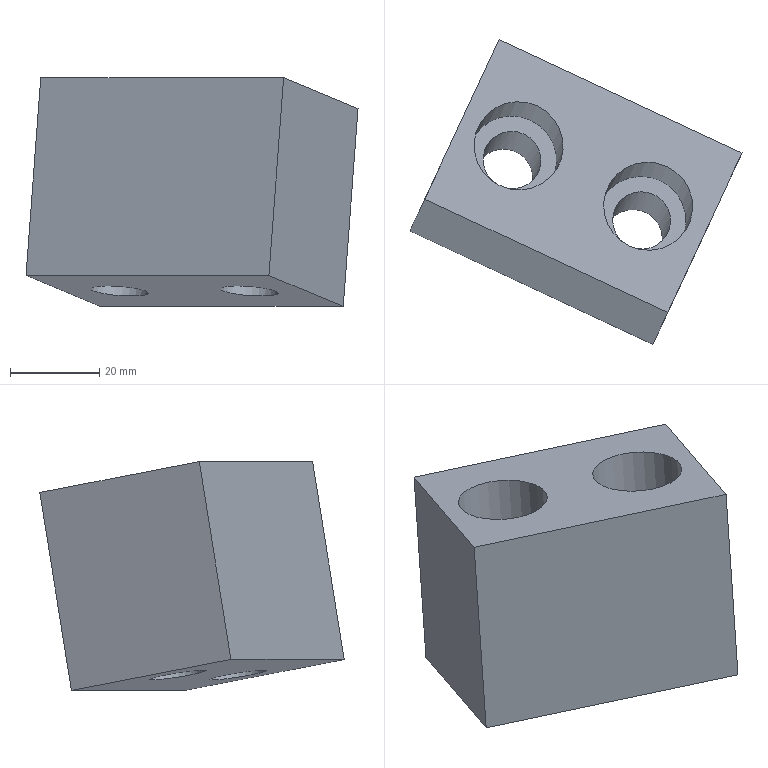Part | NX | features solid 2 | 1 solid | 12 faces | box 74.329 x 68.141 x 51.262 mm | volume 88797 mm3 | plane 8 | cylinder 4 | commonest cylinder face diameters 13 x2 20 x2
STEP:
#1=CARTESIAN_POINT('',(315.95,683.902,73.039));
#2=VERTEX_POINT('',#1);
#3=CARTESIAN_POINT('',(317.057,677.565,73.969));
#4=DIRECTION('',(-0.07339,-0.1574,-0.9848));
#5=DIRECTION('',(-0.1704,0.9749,-0.1431));
#6=AXIS2_PLACEMENT_3D('',#3,#4,#5);
#7=CIRCLE('',#6,6.5);
#8=EDGE_CURVE('',#2,#2,#7,.F.);
#9=ORIENTED_EDGE('',*,*,#8,.T.);
#10=EDGE_LOOP('',(#9));
#11=FACE_BOUND('',#10,.T.);
#12=CARTESIAN_POINT('',(286.948,697.426,73.039));
#13=VERTEX_POINT('',#12);
#14=CARTESIAN_POINT('',(288.055,691.089,73.969));
#15=DIRECTION('',(-0.07339,-0.1574,-0.9848));
#16=DIRECTION('',(-0.1704,0.9749,-0.1431));
#17=AXIS2_PLACEMENT_3D('',#14,#15,#16);
#18=CIRCLE('',#17,6.5);
#19=EDGE_CURVE('',#13,#13,#18,.F.);
#20=ORIENTED_EDGE('',*,*,#19,.T.);
#21=EDGE_LOOP('',(#20));
#22=FACE_BOUND('',#21,.T.);
#23=CARTESIAN_POINT('',(267.043,679.155,77.442));
#24=VERTEX_POINT('',#23);
#25=CARTESIAN_POINT('',(283.691,714.857,70.496));
#26=VERTEX_POINT('',#25);
#27=CARTESIAN_POINT('',(267.043,679.155,77.442));
#28=DIRECTION('',(0.4162,0.8925,-0.1736));
#29=VECTOR('',#28,1000.);
#30=LINE('',#27,#29);
#31=EDGE_CURVE('',#24,#26,#30,.T.);
#32=ORIENTED_EDGE('',*,*,#31,.T.);
#33=CARTESIAN_POINT('',(338.07,689.499,70.496));
#34=VERTEX_POINT('',#33);
#35=CARTESIAN_POINT('',(338.07,689.499,70.496));
#36=DIRECTION('',(0.9063,-0.4226,0.));
#37=VECTOR('',#36,1000.);
#38=LINE('',#35,#37);
#39=EDGE_CURVE('',#34,#26,#38,.F.);
#40=ORIENTED_EDGE('',*,*,#39,.F.);
#41=CARTESIAN_POINT('',(321.422,653.798,77.442));
#42=VERTEX_POINT('',#41);
#43=CARTESIAN_POINT('',(321.422,653.798,77.442));
#44=DIRECTION('',(-0.4162,-0.8925,0.1736));
#45=VECTOR('',#44,1000.);
#46=LINE('',#43,#45);
#47=EDGE_CURVE('',#42,#34,#46,.F.);
#48=ORIENTED_EDGE('',*,*,#47,.F.);
#49=CARTESIAN_POINT('',(321.422,653.798,77.442));
#50=DIRECTION('',(0.9063,-0.4226,0.));
#51=VECTOR('',#50,1000.);
#52=LINE('',#49,#51);
#53=EDGE_CURVE('',#42,#24,#52,.F.);
#54=ORIENTED_EDGE('',*,*,#53,.T.);
#55=EDGE_LOOP('',(#32,#40,#48,#54));
#56=FACE_BOUND('',#55,.T.);
#57=CARTESIAN_POINT('',(321.422,653.798,77.442));
#58=DIRECTION('',(-0.07339,-0.1574,-0.9848));
#59=DIRECTION('',(-0.9063,0.4226,0.));
#60=AXIS2_PLACEMENT_3D('',#57,#58,#59);
#61=PLANE('',#60);
#62=ADVANCED_FACE('',(#11,#22,#56),#61,.T.);
#63=ORIENTED_EDGE('',*,*,#47,.T.);
#64=CARTESIAN_POINT('',(341.372,696.581,114.812));
#65=VERTEX_POINT('',#64);
#66=CARTESIAN_POINT('',(336.969,687.139,55.724));
#67=DIRECTION('',(-0.07339,-0.1574,-0.9848));
#68=VECTOR('',#67,1000.);
#69=LINE('',#66,#68);
#70=EDGE_CURVE('',#34,#65,#69,.F.);
#71=ORIENTED_EDGE('',*,*,#70,.T.);
#72=CARTESIAN_POINT('',(324.724,660.88,121.758));
#73=VERTEX_POINT('',#72);
#74=CARTESIAN_POINT('',(324.724,660.88,121.758));
#75=DIRECTION('',(0.4162,0.8925,-0.1736));
#76=VECTOR('',#75,1000.);
#77=LINE('',#74,#76);
#78=EDGE_CURVE('',#73,#65,#77,.T.);
#79=ORIENTED_EDGE('',*,*,#78,.F.);
#80=CARTESIAN_POINT('',(320.321,651.437,62.67));
#81=DIRECTION('',(0.07339,0.1574,0.9848));
#82=VECTOR('',#81,1000.);
#83=LINE('',#80,#82);
#84=EDGE_CURVE('',#42,#73,#83,.T.);
#85=ORIENTED_EDGE('',*,*,#84,.F.);
#86=EDGE_LOOP('',(#63,#71,#79,#85));
#87=FACE_BOUND('',#86,.T.);
#88=CARTESIAN_POINT('',(320.321,651.437,62.67));
#89=DIRECTION('',(-0.9063,0.4226,0.));
#90=DIRECTION('',(0.07339,0.1574,0.9848));
#91=AXIS2_PLACEMENT_3D('',#88,#89,#90);
#92=PLANE('',#91);
#93=ADVANCED_FACE('',(#87),#92,.F.);
#94=CARTESIAN_POINT('',(316.198,675.722,120.022));
#95=VERTEX_POINT('',#94);
#96=CARTESIAN_POINT('',(320.36,684.647,118.285));
#97=DIRECTION('',(-0.07339,-0.1574,-0.9848));
#98=DIRECTION('',(-0.4162,-0.8925,0.1736));
#99=AXIS2_PLACEMENT_3D('',#96,#97,#98);
#100=CIRCLE('',#99,10.);
#101=EDGE_CURVE('',#95,#95,#100,.T.);
#102=ORIENTED_EDGE('',*,*,#101,.T.);
#103=EDGE_LOOP('',(#102));
#104=FACE_BOUND('',#103,.T.);
#105=CARTESIAN_POINT('',(287.196,689.246,120.022));
#106=VERTEX_POINT('',#105);
#107=CARTESIAN_POINT('',(291.358,698.171,118.285));
#108=DIRECTION('',(-0.07339,-0.1574,-0.9848));
#109=DIRECTION('',(-0.4162,-0.8925,0.1736));
#110=AXIS2_PLACEMENT_3D('',#107,#108,#109);
#111=CIRCLE('',#110,10.);
#112=EDGE_CURVE('',#106,#106,#111,.T.);
#113=ORIENTED_EDGE('',*,*,#112,.T.);
#114=EDGE_LOOP('',(#113));
#115=FACE_BOUND('',#114,.T.);
#116=ORIENTED_EDGE('',*,*,#78,.T.);
#117=CARTESIAN_POINT('',(286.993,721.939,114.812));
#118=VERTEX_POINT('',#117);
#119=CARTESIAN_POINT('',(341.372,696.581,114.812));
#120=DIRECTION('',(-0.9063,0.4226,0.));
#121=VECTOR('',#120,1000.);
#122=LINE('',#119,#121);
#123=EDGE_CURVE('',#65,#118,#122,.T.);
#124=ORIENTED_EDGE('',*,*,#123,.T.);
#125=CARTESIAN_POINT('',(270.346,686.237,121.758));
#126=VERTEX_POINT('',#125);
#127=CARTESIAN_POINT('',(270.346,686.237,121.758));
#128=DIRECTION('',(-0.4162,-0.8925,0.1736));
#129=VECTOR('',#128,1000.);
#130=LINE('',#127,#129);
#131=EDGE_CURVE('',#126,#118,#130,.F.);
#132=ORIENTED_EDGE('',*,*,#131,.F.);
#133=CARTESIAN_POINT('',(324.724,660.88,121.758));
#134=DIRECTION('',(-0.9063,0.4226,0.));
#135=VECTOR('',#134,1000.);
#136=LINE('',#133,#135);
#137=EDGE_CURVE('',#73,#126,#136,.T.);
#138=ORIENTED_EDGE('',*,*,#137,.F.);
#139=EDGE_LOOP('',(#116,#124,#132,#138));
#140=FACE_BOUND('',#139,.T.);
#141=CARTESIAN_POINT('',(324.724,660.88,121.758));
#142=DIRECTION('',(-0.07339,-0.1574,-0.9848));
#143=DIRECTION('',(-0.9063,0.4226,0.));
#144=AXIS2_PLACEMENT_3D('',#141,#142,#143);
#145=PLANE('',#144);
#146=ADVANCED_FACE('',(#104,#115,#140),#145,.F.);
#147=CARTESIAN_POINT('',(265.942,676.794,62.67));
#148=DIRECTION('',(0.07339,0.1574,0.9848));
#149=VECTOR('',#148,1000.);
#150=LINE('',#147,#149);
#151=EDGE_CURVE('',#24,#126,#150,.T.);
#152=ORIENTED_EDGE('',*,*,#151,.T.);
#153=ORIENTED_EDGE('',*,*,#131,.T.);
#154=CARTESIAN_POINT('',(282.59,712.496,55.724));
#155=DIRECTION('',(-0.07339,-0.1574,-0.9848));
#156=VECTOR('',#155,1000.);
#157=LINE('',#154,#156);
#158=EDGE_CURVE('',#26,#118,#157,.F.);
#159=ORIENTED_EDGE('',*,*,#158,.F.);
#160=ORIENTED_EDGE('',*,*,#31,.F.);
#161=EDGE_LOOP('',(#152,#153,#159,#160));
#162=FACE_BOUND('',#161,.T.);
#163=CARTESIAN_POINT('',(265.942,676.794,62.67));
#164=DIRECTION('',(-0.9063,0.4226,0.));
#165=DIRECTION('',(0.07339,0.1574,0.9848));
#166=AXIS2_PLACEMENT_3D('',#163,#164,#165);
#167=PLANE('',#166);
#168=ADVANCED_FACE('',(#162),#167,.T.);
#169=ORIENTED_EDGE('',*,*,#123,.F.);
#170=ORIENTED_EDGE('',*,*,#70,.F.);
#171=ORIENTED_EDGE('',*,*,#39,.T.);
#172=ORIENTED_EDGE('',*,*,#158,.T.);
#173=EDGE_LOOP('',(#169,#170,#171,#172));
#174=FACE_BOUND('',#173,.T.);
#175=CARTESIAN_POINT('',(336.969,687.139,55.724));
#176=DIRECTION('',(0.4162,0.8925,-0.1736));
#177=DIRECTION('',(-0.07339,-0.1574,-0.9848));
#178=AXIS2_PLACEMENT_3D('',#175,#176,#177);
#179=PLANE('',#178);
#180=ADVANCED_FACE('',(#174),#179,.T.);
#181=ORIENTED_EDGE('',*,*,#137,.T.);
#182=ORIENTED_EDGE('',*,*,#151,.F.);
#183=ORIENTED_EDGE('',*,*,#53,.F.);
#184=ORIENTED_EDGE('',*,*,#84,.T.);
#185=EDGE_LOOP('',(#181,#182,#183,#184));
#186=FACE_BOUND('',#185,.T.);
#187=CARTESIAN_POINT('',(320.321,651.437,62.67));
#188=DIRECTION('',(0.4162,0.8925,-0.1736));
#189=DIRECTION('',(-0.07339,-0.1574,-0.9848));
#190=AXIS2_PLACEMENT_3D('',#187,#188,#189);
#191=PLANE('',#190);
#192=ADVANCED_FACE('',(#186),#191,.F.);
#193=CARTESIAN_POINT('',(287.185,689.222,99.718));
#194=VERTEX_POINT('',#193);
#195=CARTESIAN_POINT('',(289.89,695.024,98.589));
#196=DIRECTION('',(-0.07339,-0.1574,-0.9848));
#197=DIRECTION('',(-0.4162,-0.8925,0.1736));
#198=AXIS2_PLACEMENT_3D('',#195,#196,#197);
#199=CIRCLE('',#198,6.5);
#200=EDGE_CURVE('',#194,#194,#199,.T.);
#201=ORIENTED_EDGE('',*,*,#200,.F.);
#202=EDGE_LOOP('',(#201));
#203=FACE_BOUND('',#202,.T.);
#204=ORIENTED_EDGE('',*,*,#19,.F.);
#205=EDGE_LOOP('',(#204));
#206=FACE_BOUND('',#205,.T.);
#207=CARTESIAN_POINT('',(285.487,685.581,39.5));
#208=DIRECTION('',(-0.07339,-0.1574,-0.9848));
#209=DIRECTION('',(-0.4162,-0.8925,0.1736));
#210=AXIS2_PLACEMENT_3D('',#207,#208,#209);
#211=CYLINDRICAL_SURFACE('',#210,6.5);
#212=ADVANCED_FACE('',(#203,#206),#211,.F.);
#213=ORIENTED_EDGE('',*,*,#200,.T.);
#214=EDGE_LOOP('',(#213));
#215=FACE_BOUND('',#214,.T.);
#216=CARTESIAN_POINT('',(285.728,686.098,100.325));
#217=VERTEX_POINT('',#216);
#218=CARTESIAN_POINT('',(289.89,695.024,98.589));
#219=DIRECTION('',(-0.07339,-0.1574,-0.9848));
#220=DIRECTION('',(-0.4162,-0.8925,0.1736));
#221=AXIS2_PLACEMENT_3D('',#218,#219,#220);
#222=CIRCLE('',#221,10.);
#223=EDGE_CURVE('',#217,#217,#222,.T.);
#224=ORIENTED_EDGE('',*,*,#223,.F.);
#225=EDGE_LOOP('',(#224));
#226=FACE_BOUND('',#225,.T.);
#227=CARTESIAN_POINT('',(288.077,695.869,98.589));
#228=DIRECTION('',(-0.07339,-0.1574,-0.9848));
#229=DIRECTION('',(-0.4162,-0.8925,0.1736));
#230=AXIS2_PLACEMENT_3D('',#227,#228,#229);
#231=PLANE('',#230);
#232=ADVANCED_FACE('',(#215,#226),#231,.F.);
#233=ORIENTED_EDGE('',*,*,#223,.T.);
#234=EDGE_LOOP('',(#233));
#235=FACE_BOUND('',#234,.T.);
#236=ORIENTED_EDGE('',*,*,#112,.F.);
#237=EDGE_LOOP('',(#236));
#238=FACE_BOUND('',#237,.T.);
#239=CARTESIAN_POINT('',(291.358,698.171,118.285));
#240=DIRECTION('',(-0.07339,-0.1574,-0.9848));
#241=DIRECTION('',(-0.4162,-0.8925,0.1736));
#242=AXIS2_PLACEMENT_3D('',#239,#240,#241);
#243=CYLINDRICAL_SURFACE('',#242,10.);
#244=ADVANCED_FACE('',(#235,#238),#243,.F.);
#245=CARTESIAN_POINT('',(316.187,675.698,99.718));
#246=VERTEX_POINT('',#245);
#247=CARTESIAN_POINT('',(318.892,681.5,98.589));
#248=DIRECTION('',(-0.07339,-0.1574,-0.9848));
#249=DIRECTION('',(-0.4162,-0.8925,0.1736));
#250=AXIS2_PLACEMENT_3D('',#247,#248,#249);
#251=CIRCLE('',#250,6.5);
#252=EDGE_CURVE('',#246,#246,#251,.T.);
#253=ORIENTED_EDGE('',*,*,#252,.F.);
#254=EDGE_LOOP('',(#253));
#255=FACE_BOUND('',#254,.T.);
#256=ORIENTED_EDGE('',*,*,#8,.F.);
#257=EDGE_LOOP('',(#256));
#258=FACE_BOUND('',#257,.T.);
#259=CARTESIAN_POINT('',(314.489,672.057,39.5));
#260=DIRECTION('',(-0.07339,-0.1574,-0.9848));
#261=DIRECTION('',(-0.4162,-0.8925,0.1736));
#262=AXIS2_PLACEMENT_3D('',#259,#260,#261);
#263=CYLINDRICAL_SURFACE('',#262,6.5);
#264=ADVANCED_FACE('',(#255,#258),#263,.F.);
#265=ORIENTED_EDGE('',*,*,#252,.T.);
#266=EDGE_LOOP('',(#265));
#267=FACE_BOUND('',#266,.T.);
#268=CARTESIAN_POINT('',(314.73,672.574,100.325));
#269=VERTEX_POINT('',#268);
#270=CARTESIAN_POINT('',(318.892,681.5,98.589));
#271=DIRECTION('',(-0.07339,-0.1574,-0.9848));
#272=DIRECTION('',(-0.4162,-0.8925,0.1736));
#273=AXIS2_PLACEMENT_3D('',#270,#271,#272);
#274=CIRCLE('',#273,10.);
#275=EDGE_CURVE('',#269,#269,#274,.T.);
#276=ORIENTED_EDGE('',*,*,#275,.F.);
#277=EDGE_LOOP('',(#276));
#278=FACE_BOUND('',#277,.T.);
#279=CARTESIAN_POINT('',(320.705,680.655,98.589));
#280=DIRECTION('',(-0.07339,-0.1574,-0.9848));
#281=DIRECTION('',(-0.4162,-0.8925,0.1736));
#282=AXIS2_PLACEMENT_3D('',#279,#280,#281);
#283=PLANE('',#282);
#284=ADVANCED_FACE('',(#267,#278),#283,.F.);
#285=ORIENTED_EDGE('',*,*,#275,.T.);
#286=EDGE_LOOP('',(#285));
#287=FACE_BOUND('',#286,.T.);
#288=ORIENTED_EDGE('',*,*,#101,.F.);
#289=EDGE_LOOP('',(#288));
#290=FACE_BOUND('',#289,.T.);
#291=CARTESIAN_POINT('',(320.36,684.647,118.285));
#292=DIRECTION('',(-0.07339,-0.1574,-0.9848));
#293=DIRECTION('',(-0.4162,-0.8925,0.1736));
#294=AXIS2_PLACEMENT_3D('',#291,#292,#293);
#295=CYLINDRICAL_SURFACE('',#294,10.);
#296=ADVANCED_FACE('',(#287,#290),#295,.F.);
#297=CLOSED_SHELL('',(#62,#93,#146,#168,#180,#192,#212,#232,#244,#264,#284,#296));
#298=MANIFOLD_SOLID_BREP('',#297);
#299=(LENGTH_UNIT()NAMED_UNIT(*)SI_UNIT(.MILLI.,.METRE.));
#300=UNCERTAINTY_MEASURE_WITH_UNIT(LENGTH_MEASURE(0.00001),#299,'','');
#301=(NAMED_UNIT(*)PLANE_ANGLE_UNIT()SI_UNIT($,.RADIAN.));
#302=(NAMED_UNIT(*)SI_UNIT($,.STERADIAN.)SOLID_ANGLE_UNIT());
#303=(GEOMETRIC_REPRESENTATION_CONTEXT(3)GLOBAL_UNCERTAINTY_ASSIGNED_CONTEXT((#300))GLOBAL_UNIT_ASSIGNED_CONTEXT((#299,#301,#302))REPRESENTATION_CONTEXT('',''));
#304=ADVANCED_BREP_SHAPE_REPRESENTATION('',(#298),#303);